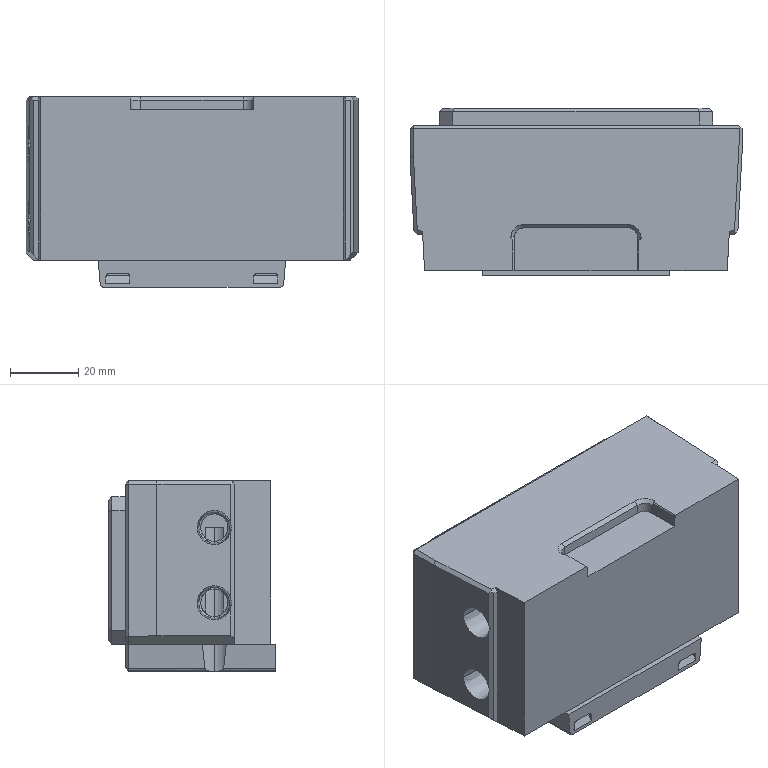Part | Creo | 1 solid | 263 faces | box 97 x 48.983 x 55.677 mm | volume 208598 mm3 | plane 119 | other 88 | cylinder 36 | cone 17 | spline 3 | commonest cylinder face diameters 8 x22 2.01 x6 10 x4 6 x2 0.6 x1 1 x1